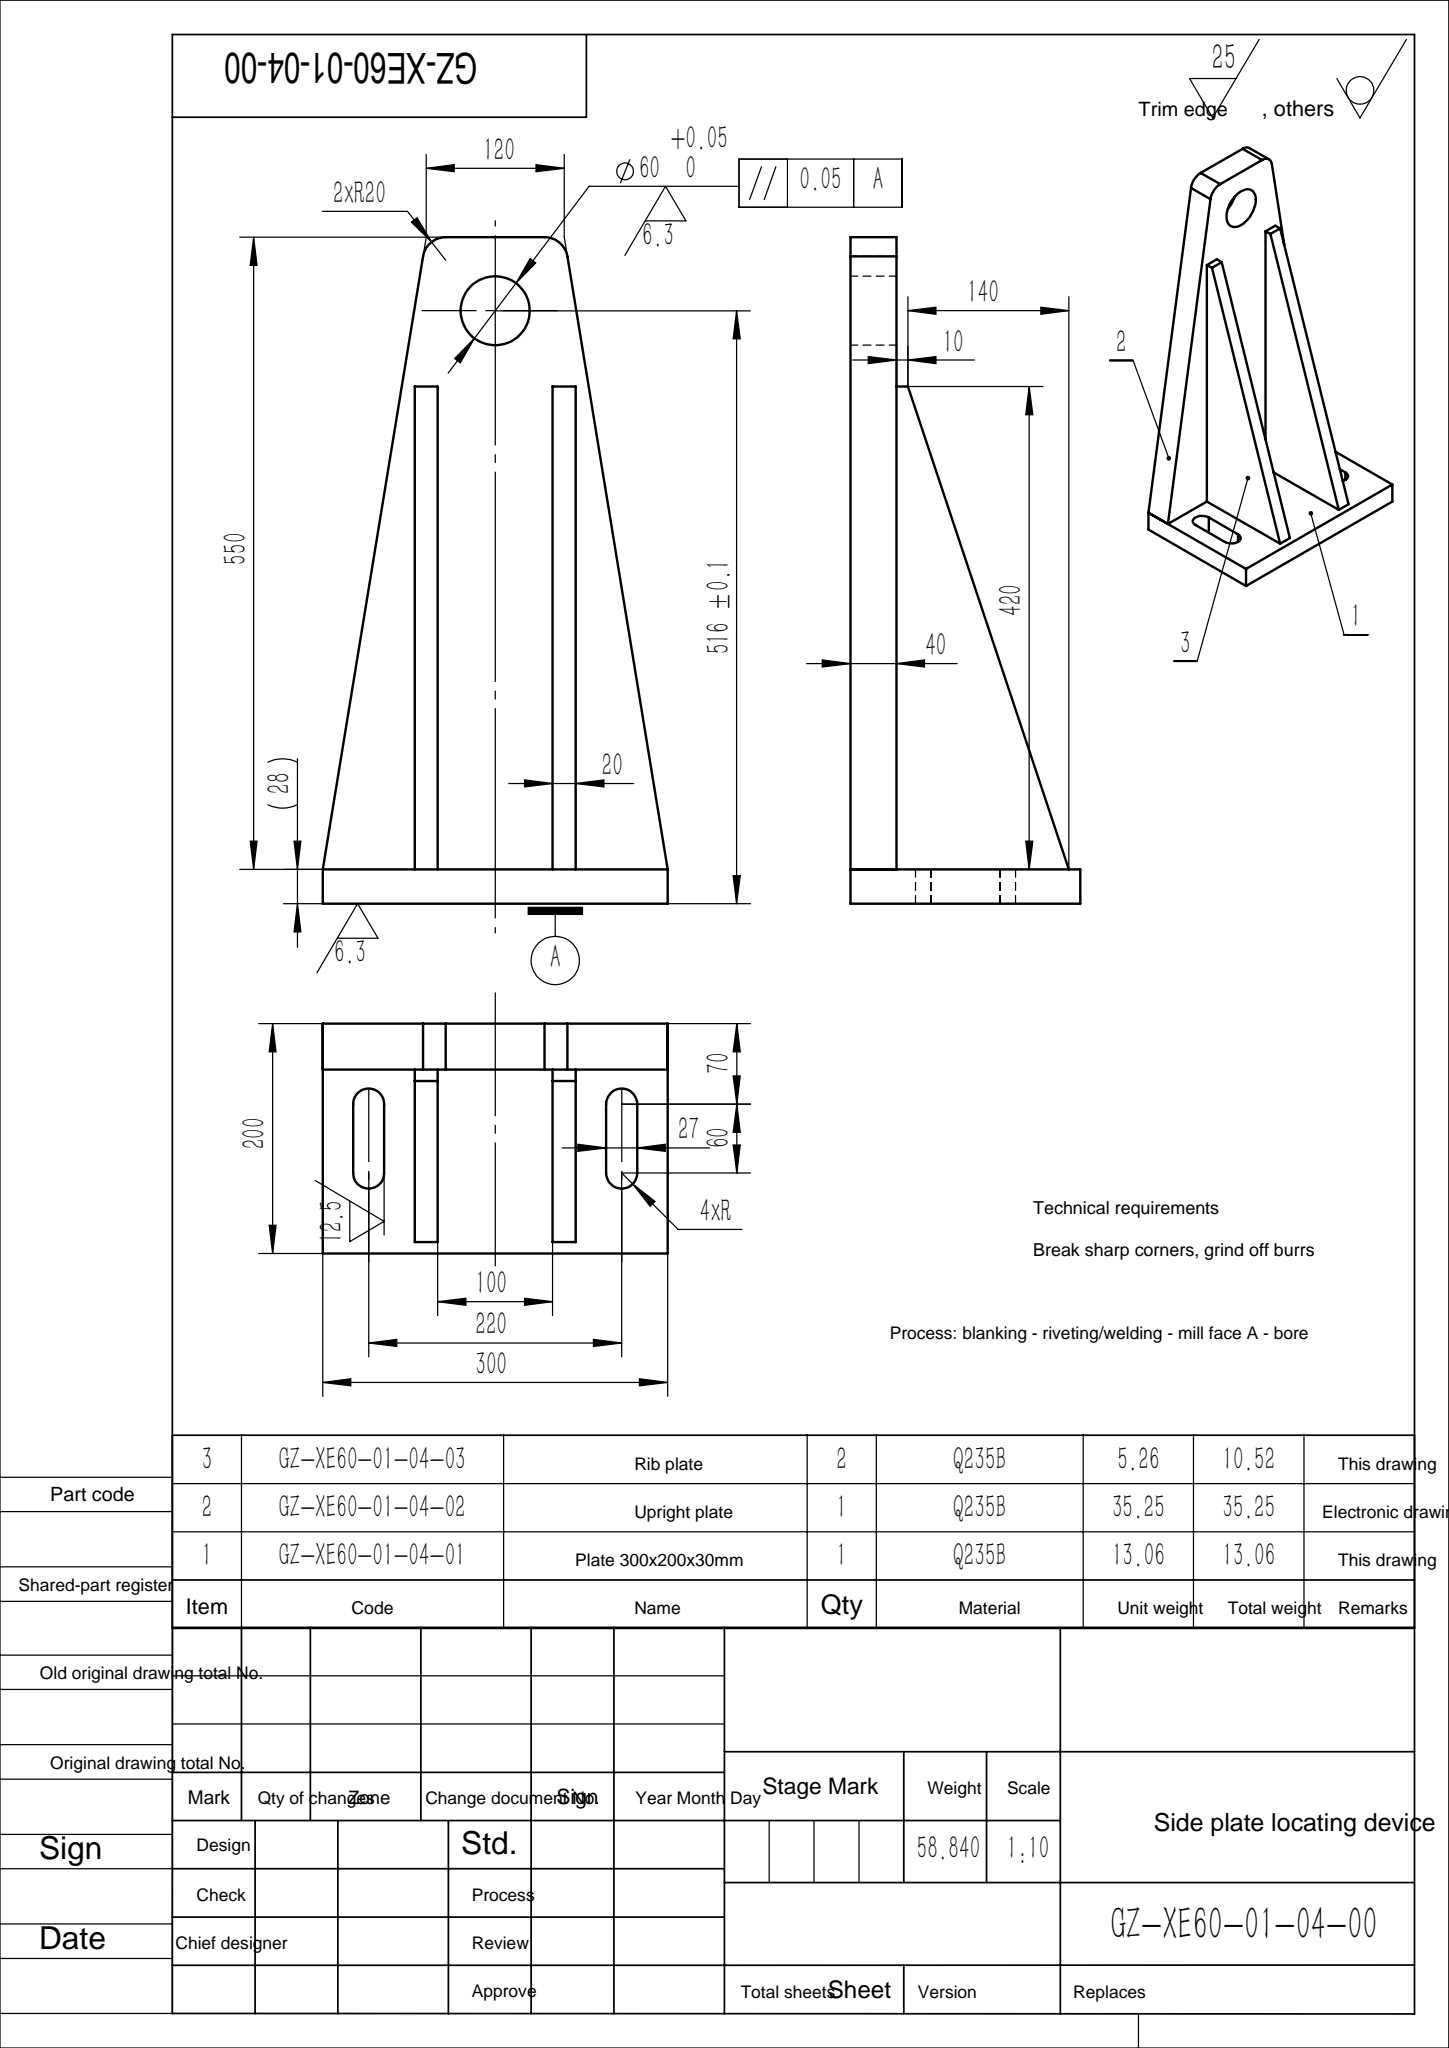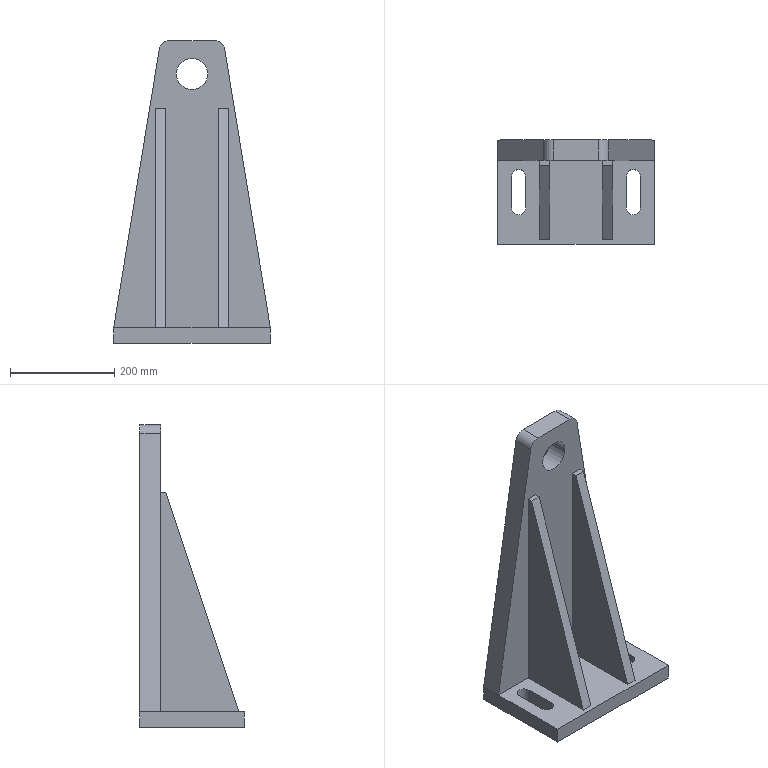Part | SolidWorks | 4 solids | 36 faces | box 300 x 200 x 580 mm | volume 7514698 mm3 | plane 28 | cylinder 8 | commonest cylinder face diameters 27 x4 40 x2 60 x2